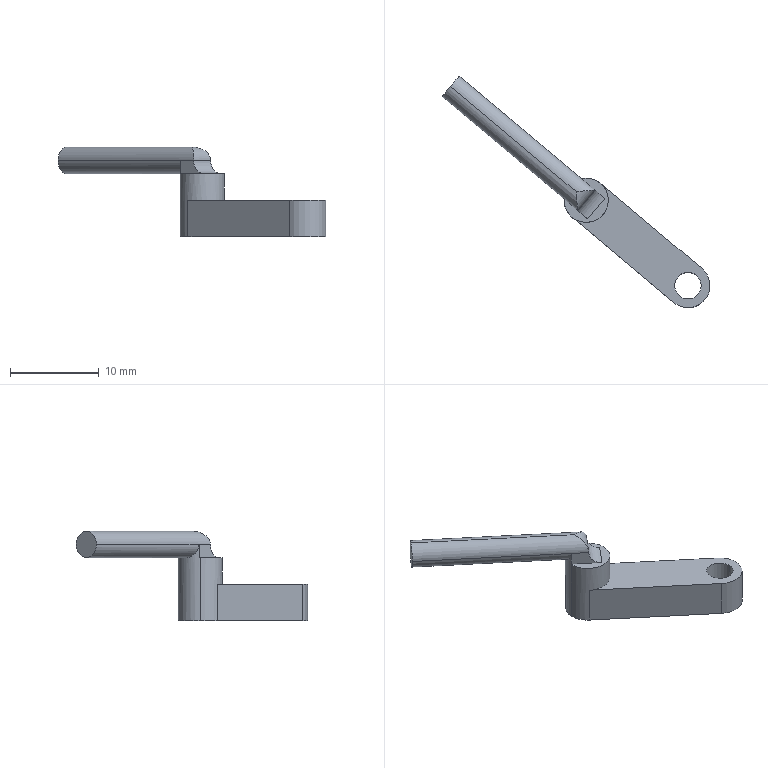Part | SolidWorks | features ICE 3, Extrusion 1, Fillet 1, MirrorPattern 1 | 1 solid | 22 faces | box 30.276 x 26.147 x 10.13 mm | volume 535.495 mm3 | cylinder 13 | plane 9 | commonest cylinder face diameters 3 x10 5 x3
STEP:
#1=CARTESIAN_POINT('',(-12.991,9.642,2.065));
#2=VERTEX_POINT('',#1);
#3=CARTESIAN_POINT('',(-9.991,9.642,2.065));
#4=VERTEX_POINT('',#3);
#5=CARTESIAN_POINT('',(-11.491,9.642,2.065));
#6=DIRECTION('',(0.,0.,1.));
#7=DIRECTION('',(1.,0.,0.));
#8=AXIS2_PLACEMENT_3D('',#5,#6,#7);
#9=CIRCLE('',#8,1.5);
#10=EDGE_CURVE('',#2,#4,#9,.T.);
#11=ORIENTED_EDGE('',*,*,#10,.T.);
#12=CARTESIAN_POINT('',(-9.991,9.642,-2.065));
#13=VERTEX_POINT('',#12);
#14=CARTESIAN_POINT('',(-9.991,9.642,2.065));
#15=DIRECTION('',(0.,0.,-1.));
#16=VECTOR('',#15,1000.);
#17=LINE('',#14,#16);
#18=EDGE_CURVE('',#4,#13,#17,.T.);
#19=ORIENTED_EDGE('',*,*,#18,.T.);
#20=CARTESIAN_POINT('',(-12.991,9.642,-2.065));
#21=VERTEX_POINT('',#20);
#22=CARTESIAN_POINT('',(-11.491,9.642,-2.065));
#23=DIRECTION('',(0.,0.,1.));
#24=DIRECTION('',(1.,0.,0.));
#25=AXIS2_PLACEMENT_3D('',#22,#23,#24);
#26=CIRCLE('',#25,1.5);
#27=EDGE_CURVE('',#21,#13,#26,.T.);
#28=ORIENTED_EDGE('',*,*,#27,.F.);
#29=CARTESIAN_POINT('',(-12.991,9.642,2.065));
#30=DIRECTION('',(0.,0.,-1.));
#31=VECTOR('',#30,1000.);
#32=LINE('',#29,#31);
#33=EDGE_CURVE('',#2,#21,#32,.T.);
#34=ORIENTED_EDGE('',*,*,#33,.F.);
#35=EDGE_LOOP('',(#11,#19,#28,#34));
#36=FACE_OUTER_BOUND('',#35,.T.);
#37=CARTESIAN_POINT('',(-11.491,9.642,2.065));
#38=DIRECTION('',(0.,0.,-1.));
#39=DIRECTION('',(-1.,0.,0.));
#40=AXIS2_PLACEMENT_3D('',#37,#38,#39);
#41=CYLINDRICAL_SURFACE('',#40,1.5);
#42=ADVANCED_FACE('',(#36),#41,.F.);
#43=CARTESIAN_POINT('',(-8.991,9.642,5.065));
#44=VERTEX_POINT('',#43);
#45=CARTESIAN_POINT('',(-12.059,12.076,5.065));
#46=VERTEX_POINT('',#45);
#47=CARTESIAN_POINT('',(-11.491,9.642,5.065));
#48=DIRECTION('',(0.,0.,1.));
#49=DIRECTION('',(1.,0.,0.));
#50=AXIS2_PLACEMENT_3D('',#47,#48,#49);
#51=CIRCLE('',#50,2.5);
#52=EDGE_CURVE('',#44,#46,#51,.T.);
#53=ORIENTED_EDGE('',*,*,#52,.F.);
#54=CARTESIAN_POINT('',(-8.991,9.642,2.065));
#55=VERTEX_POINT('',#54);
#56=CARTESIAN_POINT('',(-8.991,9.642,2.065));
#57=DIRECTION('',(0.,0.,-1.));
#58=VECTOR('',#57,1000.);
#59=LINE('',#56,#58);
#60=EDGE_CURVE('',#44,#55,#59,.T.);
#61=ORIENTED_EDGE('',*,*,#60,.T.);
#62=CARTESIAN_POINT('',(-9.884,11.557,2.065));
#63=VERTEX_POINT('',#62);
#64=CARTESIAN_POINT('',(-11.491,9.642,2.065));
#65=DIRECTION('',(0.,0.,1.));
#66=DIRECTION('',(1.,0.,0.));
#67=AXIS2_PLACEMENT_3D('',#64,#65,#66);
#68=CIRCLE('',#67,2.5);
#69=EDGE_CURVE('',#55,#63,#68,.T.);
#70=ORIENTED_EDGE('',*,*,#69,.T.);
#71=CARTESIAN_POINT('',(-9.884,11.557,-2.065));
#72=VERTEX_POINT('',#71);
#73=CARTESIAN_POINT('',(-9.884,11.557,2.065));
#74=DIRECTION('',(0.,0.,-1.));
#75=VECTOR('',#74,1000.);
#76=LINE('',#73,#75);
#77=EDGE_CURVE('',#63,#72,#76,.T.);
#78=ORIENTED_EDGE('',*,*,#77,.T.);
#79=CARTESIAN_POINT('',(-13.991,9.642,-2.065));
#80=VERTEX_POINT('',#79);
#81=CARTESIAN_POINT('',(-11.491,9.642,-2.065));
#82=DIRECTION('',(0.,0.,1.));
#83=DIRECTION('',(1.,0.,0.));
#84=AXIS2_PLACEMENT_3D('',#81,#82,#83);
#85=CIRCLE('',#84,2.5);
#86=EDGE_CURVE('',#72,#80,#85,.T.);
#87=ORIENTED_EDGE('',*,*,#86,.T.);
#88=CARTESIAN_POINT('',(-13.991,9.642,5.065));
#89=VERTEX_POINT('',#88);
#90=CARTESIAN_POINT('',(-13.991,9.642,2.065));
#91=DIRECTION('',(0.,0.,-1.));
#92=VECTOR('',#91,1000.);
#93=LINE('',#90,#92);
#94=EDGE_CURVE('',#89,#80,#93,.T.);
#95=ORIENTED_EDGE('',*,*,#94,.F.);
#96=CARTESIAN_POINT('',(-13.987,9.778,5.065));
#97=VERTEX_POINT('',#96);
#98=CARTESIAN_POINT('',(-11.491,9.642,5.065));
#99=DIRECTION('',(0.,0.,1.));
#100=DIRECTION('',(1.,0.,0.));
#101=AXIS2_PLACEMENT_3D('',#98,#99,#100);
#102=CIRCLE('',#101,2.5);
#103=EDGE_CURVE('',#97,#89,#102,.T.);
#104=ORIENTED_EDGE('',*,*,#103,.F.);
#105=CARTESIAN_POINT('',(-13.987,9.778,6.565));
#106=VERTEX_POINT('',#105);
#107=CARTESIAN_POINT('',(-13.987,9.778,6.565));
#108=DIRECTION('',(0.,0.,-1.));
#109=VECTOR('',#108,1000.);
#110=LINE('',#107,#109);
#111=EDGE_CURVE('',#106,#97,#110,.T.);
#112=ORIENTED_EDGE('',*,*,#111,.F.);
#113=CARTESIAN_POINT('',(-13.406,11.249,5.065));
#114=VERTEX_POINT('',#113);
#115=CARTESIAN_POINT('',(-13.987,9.778,6.565));
#116=CARTESIAN_POINT('',(-13.987,9.778,6.463));
#117=CARTESIAN_POINT('',(-13.986,9.791,6.363));
#118=CARTESIAN_POINT('',(-13.983,9.84,6.169));
#119=CARTESIAN_POINT('',(-13.98,9.877,6.073));
#120=CARTESIAN_POINT('',(-13.965,10.012,5.803));
#121=CARTESIAN_POINT('',(-13.945,10.139,5.641));
#122=CARTESIAN_POINT('',(-13.888,10.355,5.438));
#123=CARTESIAN_POINT('',(-13.864,10.432,5.376));
#124=CARTESIAN_POINT('',(-13.805,10.592,5.268));
#125=CARTESIAN_POINT('',(-13.77,10.673,5.222));
#126=CARTESIAN_POINT('',(-13.687,10.839,5.145));
#127=CARTESIAN_POINT('',(-13.639,10.925,5.115));
#128=CARTESIAN_POINT('',(-13.531,11.09,5.075));
#129=CARTESIAN_POINT('',(-13.471,11.171,5.065));
#130=CARTESIAN_POINT('',(-13.406,11.249,5.065));
#131=B_SPLINE_CURVE_WITH_KNOTS('',3,(#115,#116,#117,#118,#119,#120,#121,#122,#123,#124,#125,#126,#127,#128,#129,#130),.UNSPECIFIED.,.F.,.F.,(4,2,2,2,2,2,2,4),(0.,0.0003008,0.0006016,0.001203,0.001504,0.001805,0.002105,0.002406),.UNSPECIFIED.);
#132=EDGE_CURVE('',#106,#114,#131,.T.);
#133=ORIENTED_EDGE('',*,*,#132,.T.);
#134=CARTESIAN_POINT('',(-12.059,12.076,6.565));
#135=VERTEX_POINT('',#134);
#136=CARTESIAN_POINT('',(-13.406,11.249,5.065));
#137=CARTESIAN_POINT('',(-13.34,11.327,5.065));
#138=CARTESIAN_POINT('',(-13.271,11.399,5.075));
#139=CARTESIAN_POINT('',(-13.128,11.534,5.115));
#140=CARTESIAN_POINT('',(-13.052,11.597,5.145));
#141=CARTESIAN_POINT('',(-12.827,11.763,5.26));
#142=CARTESIAN_POINT('',(-12.676,11.848,5.371));
#143=CARTESIAN_POINT('',(-12.406,11.973,5.642));
#144=CARTESIAN_POINT('',(-12.285,12.014,5.803));
#145=CARTESIAN_POINT('',(-12.154,12.053,6.072));
#146=CARTESIAN_POINT('',(-12.119,12.062,6.168));
#147=CARTESIAN_POINT('',(-12.071,12.074,6.363));
#148=CARTESIAN_POINT('',(-12.059,12.076,6.463));
#149=CARTESIAN_POINT('',(-12.059,12.076,6.565));
#150=B_SPLINE_CURVE_WITH_KNOTS('',3,(#136,#137,#138,#139,#140,#141,#142,#143,#144,#145,#146,#147,#148,#149),.UNSPECIFIED.,.F.,.F.,(4,2,2,2,2,2,4),(0.,0.0003009,0.0006019,0.001204,0.001806,0.002107,0.002407),.UNSPECIFIED.);
#151=EDGE_CURVE('',#114,#135,#150,.T.);
#152=ORIENTED_EDGE('',*,*,#151,.T.);
#153=CARTESIAN_POINT('',(-12.059,12.076,5.065));
#154=DIRECTION('',(0.,0.,1.));
#155=VECTOR('',#154,1000.);
#156=LINE('',#153,#155);
#157=EDGE_CURVE('',#46,#135,#156,.T.);
#158=ORIENTED_EDGE('',*,*,#157,.F.);
#159=EDGE_LOOP('',(#53,#61,#70,#78,#87,#95,#104,#112,#133,#152,#158));
#160=FACE_OUTER_BOUND('',#159,.T.);
#161=CARTESIAN_POINT('',(-11.491,9.642,2.065));
#162=DIRECTION('',(0.,0.,-1.));
#163=DIRECTION('',(-1.,0.,0.));
#164=AXIS2_PLACEMENT_3D('',#161,#162,#163);
#165=CYLINDRICAL_SURFACE('',#164,2.5);
#166=ADVANCED_FACE('',(#160),#165,.T.);
#167=CARTESIAN_POINT('',(-1.5,0.,2.065));
#168=VERTEX_POINT('',#167);
#169=CARTESIAN_POINT('',(1.5,0.,2.065));
#170=VERTEX_POINT('',#169);
#171=CARTESIAN_POINT('',(0.,0.,2.065));
#172=DIRECTION('',(0.,0.,1.));
#173=DIRECTION('',(1.,0.,0.));
#174=AXIS2_PLACEMENT_3D('',#171,#172,#173);
#175=CIRCLE('',#174,1.5);
#176=EDGE_CURVE('',#168,#170,#175,.T.);
#177=ORIENTED_EDGE('',*,*,#176,.T.);
#178=CARTESIAN_POINT('',(1.5,0.,-2.065));
#179=VERTEX_POINT('',#178);
#180=CARTESIAN_POINT('',(1.5,0.,2.065));
#181=DIRECTION('',(0.,0.,-1.));
#182=VECTOR('',#181,1000.);
#183=LINE('',#180,#182);
#184=EDGE_CURVE('',#170,#179,#183,.T.);
#185=ORIENTED_EDGE('',*,*,#184,.T.);
#186=CARTESIAN_POINT('',(-1.5,0.,-2.065));
#187=VERTEX_POINT('',#186);
#188=CARTESIAN_POINT('',(0.,0.,-2.065));
#189=DIRECTION('',(0.,0.,1.));
#190=DIRECTION('',(1.,0.,0.));
#191=AXIS2_PLACEMENT_3D('',#188,#189,#190);
#192=CIRCLE('',#191,1.5);
#193=EDGE_CURVE('',#187,#179,#192,.T.);
#194=ORIENTED_EDGE('',*,*,#193,.F.);
#195=CARTESIAN_POINT('',(-1.5,0.,2.065));
#196=DIRECTION('',(0.,0.,-1.));
#197=VECTOR('',#196,1000.);
#198=LINE('',#195,#197);
#199=EDGE_CURVE('',#168,#187,#198,.T.);
#200=ORIENTED_EDGE('',*,*,#199,.F.);
#201=EDGE_LOOP('',(#177,#185,#194,#200));
#202=FACE_OUTER_BOUND('',#201,.T.);
#203=CARTESIAN_POINT('',(0.,0.,2.065));
#204=DIRECTION('',(0.,0.,-1.));
#205=DIRECTION('',(-1.,0.,0.));
#206=AXIS2_PLACEMENT_3D('',#203,#204,#205);
#207=CYLINDRICAL_SURFACE('',#206,1.5);
#208=ADVANCED_FACE('',(#202),#207,.F.);
#209=CARTESIAN_POINT('',(-9.377,9.827,5.065));
#210=VERTEX_POINT('',#209);
#211=CARTESIAN_POINT('',(0.9642,1.149,5.065));
#212=DIRECTION('',(0.766,-0.6428,0.));
#213=VECTOR('',#212,1000.);
#214=LINE('',#211,#213);
#215=EDGE_CURVE('',#46,#210,#214,.T.);
#216=ORIENTED_EDGE('',*,*,#215,.T.);
#217=CARTESIAN_POINT('',(-11.306,7.529,5.065));
#218=VERTEX_POINT('',#217);
#219=CARTESIAN_POINT('',(-10.342,8.678,5.065));
#220=DIRECTION('',(-0.6428,-0.766,0.));
#221=VECTOR('',#220,1000.);
#222=LINE('',#219,#221);
#223=EDGE_CURVE('',#210,#218,#222,.T.);
#224=ORIENTED_EDGE('',*,*,#223,.T.);
#225=CARTESIAN_POINT('',(-0.9642,-1.149,5.065));
#226=DIRECTION('',(0.766,-0.6428,0.));
#227=VECTOR('',#226,1000.);
#228=LINE('',#225,#227);
#229=EDGE_CURVE('',#97,#218,#228,.T.);
#230=ORIENTED_EDGE('',*,*,#229,.F.);
#231=ORIENTED_EDGE('',*,*,#103,.T.);
#232=CARTESIAN_POINT('',(-11.491,9.642,5.065));
#233=DIRECTION('',(0.,0.,1.));
#234=DIRECTION('',(1.,0.,0.));
#235=AXIS2_PLACEMENT_3D('',#232,#233,#234);
#236=CIRCLE('',#235,2.5);
#237=EDGE_CURVE('',#89,#44,#236,.T.);
#238=ORIENTED_EDGE('',*,*,#237,.T.);
#239=ORIENTED_EDGE('',*,*,#52,.T.);
#240=EDGE_LOOP('',(#216,#224,#230,#231,#238,#239));
#241=FACE_OUTER_BOUND('',#240,.T.);
#242=CARTESIAN_POINT('',(-11.491,9.642,5.065));
#243=DIRECTION('',(0.,0.,1.));
#244=DIRECTION('',(1.,0.,0.));
#245=AXIS2_PLACEMENT_3D('',#242,#243,#244);
#246=PLANE('',#245);
#247=ADVANCED_FACE('',(#241),#246,.T.);
#248=CARTESIAN_POINT('',(-13.098,7.727,-2.065));
#249=VERTEX_POINT('',#248);
#250=CARTESIAN_POINT('',(-1.607,-1.915,-2.065));
#251=VERTEX_POINT('',#250);
#252=CARTESIAN_POINT('',(-1.607,-1.915,-2.065));
#253=DIRECTION('',(0.766,-0.6428,0.));
#254=VECTOR('',#253,1000.);
#255=LINE('',#252,#254);
#256=EDGE_CURVE('',#249,#251,#255,.T.);
#257=ORIENTED_EDGE('',*,*,#256,.T.);
#258=CARTESIAN_POINT('',(-1.607,-1.915,2.065));
#259=VERTEX_POINT('',#258);
#260=CARTESIAN_POINT('',(-1.607,-1.915,2.065));
#261=DIRECTION('',(0.,0.,-1.));
#262=VECTOR('',#261,1000.);
#263=LINE('',#260,#262);
#264=EDGE_CURVE('',#259,#251,#263,.T.);
#265=ORIENTED_EDGE('',*,*,#264,.F.);
#266=CARTESIAN_POINT('',(-13.098,7.727,2.065));
#267=VERTEX_POINT('',#266);
#268=CARTESIAN_POINT('',(-1.607,-1.915,2.065));
#269=DIRECTION('',(0.766,-0.6428,0.));
#270=VECTOR('',#269,1000.);
#271=LINE('',#268,#270);
#272=EDGE_CURVE('',#267,#259,#271,.T.);
#273=ORIENTED_EDGE('',*,*,#272,.F.);
#274=CARTESIAN_POINT('',(-13.098,7.727,2.065));
#275=DIRECTION('',(0.,0.,-1.));
#276=VECTOR('',#275,1000.);
#277=LINE('',#274,#276);
#278=EDGE_CURVE('',#267,#249,#277,.T.);
#279=ORIENTED_EDGE('',*,*,#278,.T.);
#280=EDGE_LOOP('',(#257,#265,#273,#279));
#281=FACE_OUTER_BOUND('',#280,.T.);
#282=CARTESIAN_POINT('',(-1.607,-1.915,2.065));
#283=DIRECTION('',(0.6428,0.766,0.));
#284=DIRECTION('',(-0.766,0.6428,0.));
#285=AXIS2_PLACEMENT_3D('',#282,#283,#284);
#286=PLANE('',#285);
#287=ADVANCED_FACE('',(#281),#286,.F.);
#288=CARTESIAN_POINT('',(1.607,1.915,-2.065));
#289=VERTEX_POINT('',#288);
#290=CARTESIAN_POINT('',(0.,0.,-2.065));
#291=DIRECTION('',(0.,0.,1.));
#292=DIRECTION('',(1.,0.,0.));
#293=AXIS2_PLACEMENT_3D('',#290,#291,#292);
#294=CIRCLE('',#293,2.5);
#295=EDGE_CURVE('',#251,#289,#294,.T.);
#296=ORIENTED_EDGE('',*,*,#295,.T.);
#297=CARTESIAN_POINT('',(1.607,1.915,2.065));
#298=VERTEX_POINT('',#297);
#299=CARTESIAN_POINT('',(1.607,1.915,2.065));
#300=DIRECTION('',(0.,0.,-1.));
#301=VECTOR('',#300,1000.);
#302=LINE('',#299,#301);
#303=EDGE_CURVE('',#298,#289,#302,.T.);
#304=ORIENTED_EDGE('',*,*,#303,.F.);
#305=CARTESIAN_POINT('',(0.,0.,2.065));
#306=DIRECTION('',(0.,0.,1.));
#307=DIRECTION('',(1.,0.,0.));
#308=AXIS2_PLACEMENT_3D('',#305,#306,#307);
#309=CIRCLE('',#308,2.5);
#310=EDGE_CURVE('',#259,#298,#309,.T.);
#311=ORIENTED_EDGE('',*,*,#310,.F.);
#312=ORIENTED_EDGE('',*,*,#264,.T.);
#313=EDGE_LOOP('',(#296,#304,#311,#312));
#314=FACE_OUTER_BOUND('',#313,.T.);
#315=CARTESIAN_POINT('',(0.,0.,2.065));
#316=DIRECTION('',(0.,0.,-1.));
#317=DIRECTION('',(-1.,0.,0.));
#318=AXIS2_PLACEMENT_3D('',#315,#316,#317);
#319=CYLINDRICAL_SURFACE('',#318,2.5);
#320=ADVANCED_FACE('',(#314),#319,.T.);
#321=CARTESIAN_POINT('',(1.607,1.915,-2.065));
#322=DIRECTION('',(-0.766,0.6428,0.));
#323=VECTOR('',#322,1000.);
#324=LINE('',#321,#323);
#325=EDGE_CURVE('',#289,#72,#324,.T.);
#326=ORIENTED_EDGE('',*,*,#325,.T.);
#327=ORIENTED_EDGE('',*,*,#77,.F.);
#328=CARTESIAN_POINT('',(1.607,1.915,2.065));
#329=DIRECTION('',(-0.766,0.6428,0.));
#330=VECTOR('',#329,1000.);
#331=LINE('',#328,#330);
#332=EDGE_CURVE('',#298,#63,#331,.T.);
#333=ORIENTED_EDGE('',*,*,#332,.F.);
#334=ORIENTED_EDGE('',*,*,#303,.T.);
#335=EDGE_LOOP('',(#326,#327,#333,#334));
#336=FACE_OUTER_BOUND('',#335,.T.);
#337=CARTESIAN_POINT('',(1.607,1.915,2.065));
#338=DIRECTION('',(-0.6428,-0.766,0.));
#339=DIRECTION('',(0.766,-0.6428,0.));
#340=AXIS2_PLACEMENT_3D('',#337,#338,#339);
#341=PLANE('',#340);
#342=ADVANCED_FACE('',(#336),#341,.F.);
#343=ORIENTED_EDGE('',*,*,#184,.F.);
#344=CARTESIAN_POINT('',(0.,0.,2.065));
#345=DIRECTION('',(0.,0.,1.));
#346=DIRECTION('',(1.,0.,0.));
#347=AXIS2_PLACEMENT_3D('',#344,#345,#346);
#348=CIRCLE('',#347,1.5);
#349=EDGE_CURVE('',#170,#168,#348,.T.);
#350=ORIENTED_EDGE('',*,*,#349,.T.);
#351=ORIENTED_EDGE('',*,*,#199,.T.);
#352=CARTESIAN_POINT('',(0.,0.,-2.065));
#353=DIRECTION('',(0.,0.,1.));
#354=DIRECTION('',(1.,0.,0.));
#355=AXIS2_PLACEMENT_3D('',#352,#353,#354);
#356=CIRCLE('',#355,1.5);
#357=EDGE_CURVE('',#179,#187,#356,.T.);
#358=ORIENTED_EDGE('',*,*,#357,.F.);
#359=EDGE_LOOP('',(#343,#350,#351,#358));
#360=FACE_OUTER_BOUND('',#359,.T.);
#361=CARTESIAN_POINT('',(0.,0.,2.065));
#362=DIRECTION('',(0.,0.,-1.));
#363=DIRECTION('',(-1.,0.,0.));
#364=AXIS2_PLACEMENT_3D('',#361,#362,#363);
#365=CYLINDRICAL_SURFACE('',#364,1.5);
#366=ADVANCED_FACE('',(#360),#365,.F.);
#367=ORIENTED_EDGE('',*,*,#60,.F.);
#368=ORIENTED_EDGE('',*,*,#237,.F.);
#369=ORIENTED_EDGE('',*,*,#94,.T.);
#370=CARTESIAN_POINT('',(-11.491,9.642,-2.065));
#371=DIRECTION('',(0.,0.,1.));
#372=DIRECTION('',(1.,0.,0.));
#373=AXIS2_PLACEMENT_3D('',#370,#371,#372);
#374=CIRCLE('',#373,2.5);
#375=EDGE_CURVE('',#80,#249,#374,.T.);
#376=ORIENTED_EDGE('',*,*,#375,.T.);
#377=ORIENTED_EDGE('',*,*,#278,.F.);
#378=CARTESIAN_POINT('',(-11.491,9.642,2.065));
#379=DIRECTION('',(0.,0.,1.));
#380=DIRECTION('',(1.,0.,0.));
#381=AXIS2_PLACEMENT_3D('',#378,#379,#380);
#382=CIRCLE('',#381,2.5);
#383=EDGE_CURVE('',#267,#55,#382,.T.);
#384=ORIENTED_EDGE('',*,*,#383,.T.);
#385=EDGE_LOOP('',(#367,#368,#369,#376,#377,#384));
#386=FACE_OUTER_BOUND('',#385,.T.);
#387=CARTESIAN_POINT('',(-11.491,9.642,2.065));
#388=DIRECTION('',(0.,0.,-1.));
#389=DIRECTION('',(-1.,0.,0.));
#390=AXIS2_PLACEMENT_3D('',#387,#388,#389);
#391=CYLINDRICAL_SURFACE('',#390,2.5);
#392=ADVANCED_FACE('',(#386),#391,.T.);
#393=ORIENTED_EDGE('',*,*,#18,.F.);
#394=CARTESIAN_POINT('',(-11.491,9.642,2.065));
#395=DIRECTION('',(0.,0.,1.));
#396=DIRECTION('',(1.,0.,0.));
#397=AXIS2_PLACEMENT_3D('',#394,#395,#396);
#398=CIRCLE('',#397,1.5);
#399=EDGE_CURVE('',#4,#2,#398,.T.);
#400=ORIENTED_EDGE('',*,*,#399,.T.);
#401=ORIENTED_EDGE('',*,*,#33,.T.);
#402=CARTESIAN_POINT('',(-11.491,9.642,-2.065));
#403=DIRECTION('',(0.,0.,1.));
#404=DIRECTION('',(1.,0.,0.));
#405=AXIS2_PLACEMENT_3D('',#402,#403,#404);
#406=CIRCLE('',#405,1.5);
#407=EDGE_CURVE('',#13,#21,#406,.T.);
#408=ORIENTED_EDGE('',*,*,#407,.F.);
#409=EDGE_LOOP('',(#393,#400,#401,#408));
#410=FACE_OUTER_BOUND('',#409,.T.);
#411=CARTESIAN_POINT('',(-11.491,9.642,2.065));
#412=DIRECTION('',(0.,0.,-1.));
#413=DIRECTION('',(-1.,0.,0.));
#414=AXIS2_PLACEMENT_3D('',#411,#412,#413);
#415=CYLINDRICAL_SURFACE('',#414,1.5);
#416=ADVANCED_FACE('',(#410),#415,.F.);
#417=ORIENTED_EDGE('',*,*,#383,.F.);
#418=ORIENTED_EDGE('',*,*,#272,.T.);
#419=ORIENTED_EDGE('',*,*,#310,.T.);
#420=ORIENTED_EDGE('',*,*,#332,.T.);
#421=ORIENTED_EDGE('',*,*,#69,.F.);
#422=EDGE_LOOP('',(#417,#418,#419,#420,#421));
#423=FACE_OUTER_BOUND('',#422,.T.);
#424=ORIENTED_EDGE('',*,*,#176,.F.);
#425=ORIENTED_EDGE('',*,*,#349,.F.);
#426=EDGE_LOOP('',(#424,#425));
#427=FACE_BOUND('',#426,.T.);
#428=CARTESIAN_POINT('',(0.,0.,2.065));
#429=DIRECTION('',(0.,0.,1.));
#430=DIRECTION('',(1.,0.,0.));
#431=AXIS2_PLACEMENT_3D('',#428,#429,#430);
#432=PLANE('',#431);
#433=ADVANCED_FACE('',(#423,#427),#432,.T.);
#434=ORIENTED_EDGE('',*,*,#256,.F.);
#435=ORIENTED_EDGE('',*,*,#375,.F.);
#436=ORIENTED_EDGE('',*,*,#86,.F.);
#437=ORIENTED_EDGE('',*,*,#325,.F.);
#438=ORIENTED_EDGE('',*,*,#295,.F.);
#439=EDGE_LOOP('',(#434,#435,#436,#437,#438));
#440=FACE_OUTER_BOUND('',#439,.T.);
#441=ORIENTED_EDGE('',*,*,#193,.T.);
#442=ORIENTED_EDGE('',*,*,#357,.T.);
#443=EDGE_LOOP('',(#441,#442));
#444=FACE_BOUND('',#443,.T.);
#445=ORIENTED_EDGE('',*,*,#27,.T.);
#446=ORIENTED_EDGE('',*,*,#407,.T.);
#447=EDGE_LOOP('',(#445,#446));
#448=FACE_BOUND('',#447,.T.);
#449=CARTESIAN_POINT('',(0.,0.,-2.065));
#450=DIRECTION('',(0.,0.,1.));
#451=DIRECTION('',(1.,0.,0.));
#452=AXIS2_PLACEMENT_3D('',#449,#450,#451);
#453=PLANE('',#452);
#454=ADVANCED_FACE('',(#440,#444,#448),#453,.F.);
#455=ORIENTED_EDGE('',*,*,#10,.F.);
#456=ORIENTED_EDGE('',*,*,#399,.F.);
#457=EDGE_LOOP('',(#455,#456));
#458=FACE_OUTER_BOUND('',#457,.T.);
#459=CARTESIAN_POINT('',(-11.491,9.642,2.065));
#460=DIRECTION('',(0.,0.,1.));
#461=DIRECTION('',(1.,0.,0.));
#462=AXIS2_PLACEMENT_3D('',#459,#460,#461);
#463=PLANE('',#462);
#464=ADVANCED_FACE('',(#458),#463,.F.);
#465=ORIENTED_EDGE('',*,*,#215,.F.);
#466=ORIENTED_EDGE('',*,*,#157,.T.);
#467=CARTESIAN_POINT('',(-10.526,10.791,6.565));
#468=VERTEX_POINT('',#467);
#469=CARTESIAN_POINT('',(0.9642,1.149,6.565));
#470=DIRECTION('',(0.766,-0.6428,0.));
#471=VECTOR('',#470,1000.);
#472=LINE('',#469,#471);
#473=EDGE_CURVE('',#135,#468,#472,.T.);
#474=ORIENTED_EDGE('',*,*,#473,.T.);
#475=CARTESIAN_POINT('',(-9.377,9.827,6.565));
#476=DIRECTION('',(-0.6428,-0.766,0.));
#477=DIRECTION('',(-0.766,0.6428,0.));
#478=AXIS2_PLACEMENT_3D('',#475,#476,#477);
#479=CIRCLE('',#478,1.5);
#480=EDGE_CURVE('',#468,#210,#479,.T.);
#481=ORIENTED_EDGE('',*,*,#480,.T.);
#482=EDGE_LOOP('',(#465,#466,#474,#481));
#483=FACE_OUTER_BOUND('',#482,.T.);
#484=CARTESIAN_POINT('',(0.9642,1.149,8.065));
#485=DIRECTION('',(0.6428,0.766,0.));
#486=DIRECTION('',(-0.766,0.6428,0.));
#487=AXIS2_PLACEMENT_3D('',#484,#485,#486);
#488=PLANE('',#487);
#489=ADVANCED_FACE('',(#483),#488,.T.);
#490=CARTESIAN_POINT('',(-12.455,8.493,6.565));
#491=VERTEX_POINT('',#490);
#492=CARTESIAN_POINT('',(-27.776,21.348,6.565));
#493=DIRECTION('',(-0.766,0.6428,0.));
#494=VECTOR('',#493,1000.);
#495=LINE('',#492,#494);
#496=EDGE_CURVE('',#491,#106,#495,.T.);
#497=ORIENTED_EDGE('',*,*,#496,.T.);
#498=ORIENTED_EDGE('',*,*,#111,.T.);
#499=ORIENTED_EDGE('',*,*,#229,.T.);
#500=CARTESIAN_POINT('',(-11.306,7.529,6.565));
#501=DIRECTION('',(0.6428,0.766,0.));
#502=DIRECTION('',(-0.766,0.6428,0.));
#503=AXIS2_PLACEMENT_3D('',#500,#501,#502);
#504=CIRCLE('',#503,1.5);
#505=EDGE_CURVE('',#218,#491,#504,.T.);
#506=ORIENTED_EDGE('',*,*,#505,.T.);
#507=EDGE_LOOP('',(#497,#498,#499,#506));
#508=FACE_OUTER_BOUND('',#507,.T.);
#509=CARTESIAN_POINT('',(-0.9642,-1.149,8.065));
#510=DIRECTION('',(0.6428,0.766,0.));
#511=DIRECTION('',(-0.766,0.6428,0.));
#512=AXIS2_PLACEMENT_3D('',#509,#510,#511);
#513=PLANE('',#512);
#514=ADVANCED_FACE('',(#508),#513,.F.);
#515=CARTESIAN_POINT('',(-26.812,22.498,8.065));
#516=VERTEX_POINT('',#515);
#517=CARTESIAN_POINT('',(-25.847,23.647,6.565));
#518=VERTEX_POINT('',#517);
#519=CARTESIAN_POINT('',(-26.812,22.498,6.565));
#520=DIRECTION('',(-0.766,0.6428,0.));
#521=DIRECTION('',(0.6428,0.766,0.));
#522=AXIS2_PLACEMENT_3D('',#519,#520,#521);
#523=CIRCLE('',#522,1.5);
#524=EDGE_CURVE('',#516,#518,#523,.T.);
#525=ORIENTED_EDGE('',*,*,#524,.T.);
#526=CARTESIAN_POINT('',(-26.812,22.498,5.065));
#527=VERTEX_POINT('',#526);
#528=CARTESIAN_POINT('',(-26.812,22.498,6.565));
#529=DIRECTION('',(-0.766,0.6428,0.));
#530=DIRECTION('',(0.6428,0.766,0.));
#531=AXIS2_PLACEMENT_3D('',#528,#529,#530);
#532=CIRCLE('',#531,1.5);
#533=EDGE_CURVE('',#518,#527,#532,.T.);
#534=ORIENTED_EDGE('',*,*,#533,.T.);
#535=CARTESIAN_POINT('',(-27.776,21.348,6.565));
#536=VERTEX_POINT('',#535);
#537=CARTESIAN_POINT('',(-26.812,22.498,6.565));
#538=DIRECTION('',(-0.766,0.6428,0.));
#539=DIRECTION('',(0.6428,0.766,0.));
#540=AXIS2_PLACEMENT_3D('',#537,#538,#539);
#541=CIRCLE('',#540,1.5);
#542=EDGE_CURVE('',#527,#536,#541,.T.);
#543=ORIENTED_EDGE('',*,*,#542,.T.);
#544=CARTESIAN_POINT('',(-26.812,22.498,6.565));
#545=DIRECTION('',(-0.766,0.6428,0.));
#546=DIRECTION('',(0.6428,0.766,0.));
#547=AXIS2_PLACEMENT_3D('',#544,#545,#546);
#548=CIRCLE('',#547,1.5);
#549=EDGE_CURVE('',#536,#516,#548,.T.);
#550=ORIENTED_EDGE('',*,*,#549,.T.);
#551=EDGE_LOOP('',(#525,#534,#543,#550));
#552=FACE_OUTER_BOUND('',#551,.T.);
#553=CARTESIAN_POINT('',(-26.812,22.498,8.065));
#554=DIRECTION('',(0.766,-0.6428,0.));
#555=DIRECTION('',(0.6428,0.766,0.));
#556=AXIS2_PLACEMENT_3D('',#553,#554,#555);
#557=PLANE('',#556);
#558=ADVANCED_FACE('',(#552),#557,.F.);
#559=CARTESIAN_POINT('',(-0.9642,-1.149,6.565));
#560=DIRECTION('',(0.766,-0.6428,0.));
#561=VECTOR('',#560,1000.);
#562=LINE('',#559,#561);
#563=EDGE_CURVE('',#536,#106,#562,.T.);
#564=ORIENTED_EDGE('',*,*,#563,.F.);
#565=ORIENTED_EDGE('',*,*,#542,.F.);
#566=CARTESIAN_POINT('',(0.,0.,5.065));
#567=DIRECTION('',(-0.766,0.6428,0.));
#568=VECTOR('',#567,1000.);
#569=LINE('',#566,#568);
#570=EDGE_CURVE('',#114,#527,#569,.T.);
#571=ORIENTED_EDGE('',*,*,#570,.F.);
#572=ORIENTED_EDGE('',*,*,#132,.F.);
#573=EDGE_LOOP('',(#564,#565,#571,#572));
#574=FACE_OUTER_BOUND('',#573,.T.);
#575=CARTESIAN_POINT('',(0.,0.,6.565));
#576=DIRECTION('',(0.766,-0.6428,0.));
#577=DIRECTION('',(0.6428,0.766,0.));
#578=AXIS2_PLACEMENT_3D('',#575,#576,#577);
#579=CYLINDRICAL_SURFACE('',#578,1.5);
#580=ADVANCED_FACE('',(#574),#579,.T.);
#581=ORIENTED_EDGE('',*,*,#570,.T.);
#582=ORIENTED_EDGE('',*,*,#533,.F.);
#583=CARTESIAN_POINT('',(-25.847,23.647,6.565));
#584=DIRECTION('',(-0.766,0.6428,0.));
#585=VECTOR('',#584,1000.);
#586=LINE('',#583,#585);
#587=EDGE_CURVE('',#135,#518,#586,.T.);
#588=ORIENTED_EDGE('',*,*,#587,.F.);
#589=ORIENTED_EDGE('',*,*,#151,.F.);
#590=EDGE_LOOP('',(#581,#582,#588,#589));
#591=FACE_OUTER_BOUND('',#590,.T.);
#592=CARTESIAN_POINT('',(0.,0.,6.565));
#593=DIRECTION('',(-0.766,0.6428,0.));
#594=DIRECTION('',(-0.6428,-0.766,0.));
#595=AXIS2_PLACEMENT_3D('',#592,#593,#594);
#596=CYLINDRICAL_SURFACE('',#595,1.5);
#597=ADVANCED_FACE('',(#591),#596,.T.);
#598=ORIENTED_EDGE('',*,*,#223,.F.);
#599=ORIENTED_EDGE('',*,*,#480,.F.);
#600=CARTESIAN_POINT('',(-12.455,8.493,6.565));
#601=DIRECTION('',(0.6428,0.766,0.));
#602=VECTOR('',#601,1000.);
#603=LINE('',#600,#602);
#604=EDGE_CURVE('',#491,#468,#603,.T.);
#605=ORIENTED_EDGE('',*,*,#604,.F.);
#606=ORIENTED_EDGE('',*,*,#505,.F.);
#607=EDGE_LOOP('',(#598,#599,#605,#606));
#608=FACE_OUTER_BOUND('',#607,.T.);
#609=CARTESIAN_POINT('',(-11.306,7.529,6.565));
#610=DIRECTION('',(0.6428,0.766,0.));
#611=DIRECTION('',(-0.766,0.6428,0.));
#612=AXIS2_PLACEMENT_3D('',#609,#610,#611);
#613=CYLINDRICAL_SURFACE('',#612,1.5);
#614=ADVANCED_FACE('',(#608),#613,.F.);
#615=CARTESIAN_POINT('',(-12.64,10.606,8.065));
#616=VERTEX_POINT('',#615);
#617=CARTESIAN_POINT('',(-11.491,9.642,8.065));
#618=DIRECTION('',(0.766,-0.6428,0.));
#619=VECTOR('',#618,1000.);
#620=LINE('',#617,#619);
#621=EDGE_CURVE('',#516,#616,#620,.T.);
#622=ORIENTED_EDGE('',*,*,#621,.F.);
#623=ORIENTED_EDGE('',*,*,#549,.F.);
#624=ORIENTED_EDGE('',*,*,#563,.T.);
#625=ORIENTED_EDGE('',*,*,#496,.F.);
#626=CARTESIAN_POINT('',(-12.64,10.606,8.065));
#627=CARTESIAN_POINT('',(-12.531,9.368,8.065));
#628=CARTESIAN_POINT('',(-12.455,8.493,7.444));
#629=CARTESIAN_POINT('',(-12.455,8.493,6.565));
#630=(BOUNDED_CURVE()B_SPLINE_CURVE(3,(#626,#627,#628,#629),.UNSPECIFIED.,.F.,.F.)B_SPLINE_CURVE_WITH_KNOTS((4,4),(1.571,3.142),.UNSPECIFIED.)CURVE()GEOMETRIC_REPRESENTATION_ITEM()RATIONAL_B_SPLINE_CURVE((1.,0.8047,0.8047,1.))REPRESENTATION_ITEM(''));
#631=EDGE_CURVE('',#616,#491,#630,.T.);
#632=ORIENTED_EDGE('',*,*,#631,.F.);
#633=EDGE_LOOP('',(#622,#623,#624,#625,#632));
#634=FACE_OUTER_BOUND('',#633,.T.);
#635=CARTESIAN_POINT('',(0.,0.,6.565));
#636=DIRECTION('',(-0.766,0.6428,0.));
#637=DIRECTION('',(-0.6428,-0.766,0.));
#638=AXIS2_PLACEMENT_3D('',#635,#636,#637);
#639=CYLINDRICAL_SURFACE('',#638,1.5);
#640=ADVANCED_FACE('',(#634),#639,.T.);
#641=ORIENTED_EDGE('',*,*,#524,.F.);
#642=ORIENTED_EDGE('',*,*,#621,.T.);
#643=CARTESIAN_POINT('',(-10.526,10.791,6.565));
#644=CARTESIAN_POINT('',(-10.526,10.791,7.444));
#645=CARTESIAN_POINT('',(-11.402,10.714,8.065));
#646=CARTESIAN_POINT('',(-12.64,10.606,8.065));
#647=(BOUNDED_CURVE()B_SPLINE_CURVE(3,(#643,#644,#645,#646),.UNSPECIFIED.,.F.,.F.)B_SPLINE_CURVE_WITH_KNOTS((4,4),(0.,1.571),.UNSPECIFIED.)CURVE()GEOMETRIC_REPRESENTATION_ITEM()RATIONAL_B_SPLINE_CURVE((1.,0.8047,0.8047,1.))REPRESENTATION_ITEM(''));
#648=EDGE_CURVE('',#468,#616,#647,.T.);
#649=ORIENTED_EDGE('',*,*,#648,.F.);
#650=ORIENTED_EDGE('',*,*,#473,.F.);
#651=ORIENTED_EDGE('',*,*,#587,.T.);
#652=EDGE_LOOP('',(#641,#642,#649,#650,#651));
#653=FACE_OUTER_BOUND('',#652,.T.);
#654=CARTESIAN_POINT('',(0.,0.,6.565));
#655=DIRECTION('',(0.766,-0.6428,0.));
#656=DIRECTION('',(0.6428,0.766,0.));
#657=AXIS2_PLACEMENT_3D('',#654,#655,#656);
#658=CYLINDRICAL_SURFACE('',#657,1.5);
#659=ADVANCED_FACE('',(#653),#658,.T.);
#660=ORIENTED_EDGE('',*,*,#631,.T.);
#661=ORIENTED_EDGE('',*,*,#604,.T.);
#662=ORIENTED_EDGE('',*,*,#648,.T.);
#663=EDGE_LOOP('',(#660,#661,#662));
#664=FACE_OUTER_BOUND('',#663,.T.);
#665=CARTESIAN_POINT('',(-12.64,10.606,6.565));
#666=DIRECTION('',(-0.6428,-0.766,0.));
#667=DIRECTION('',(0.766,-0.6428,0.));
#668=AXIS2_PLACEMENT_3D('',#665,#666,#667);
#669=CYLINDRICAL_SURFACE('',#668,1.5);
#670=ADVANCED_FACE('',(#664),#669,.T.);
#671=CLOSED_SHELL('',(#42,#166,#208,#247,#287,#320,#342,#366,#392,#416,#433,#454,#464,#489,#514,#558,#580,#597,#614,#640,#659,#670));
#672=MANIFOLD_SOLID_BREP('',#671);
#673=CARTESIAN_POINT('',(0.,0.,0.));
#674=DIRECTION('',(0.,0.,1.));
#675=DIRECTION('',(1.,0.,0.));
#676=AXIS2_PLACEMENT_3D('',#673,#674,#675);
#677=(LENGTH_UNIT()NAMED_UNIT(*)SI_UNIT(.MILLI.,.METRE.));
#678=UNCERTAINTY_MEASURE_WITH_UNIT(LENGTH_MEASURE(0.00001),#677,'','');
#679=(NAMED_UNIT(*)PLANE_ANGLE_UNIT()SI_UNIT($,.RADIAN.));
#680=(NAMED_UNIT(*)SI_UNIT($,.STERADIAN.)SOLID_ANGLE_UNIT());
#681=(GEOMETRIC_REPRESENTATION_CONTEXT(3)GLOBAL_UNCERTAINTY_ASSIGNED_CONTEXT((#678))GLOBAL_UNIT_ASSIGNED_CONTEXT((#677,#679,#680))REPRESENTATION_CONTEXT('',''));
#682=ADVANCED_BREP_SHAPE_REPRESENTATION('',(#672,#676),#681);